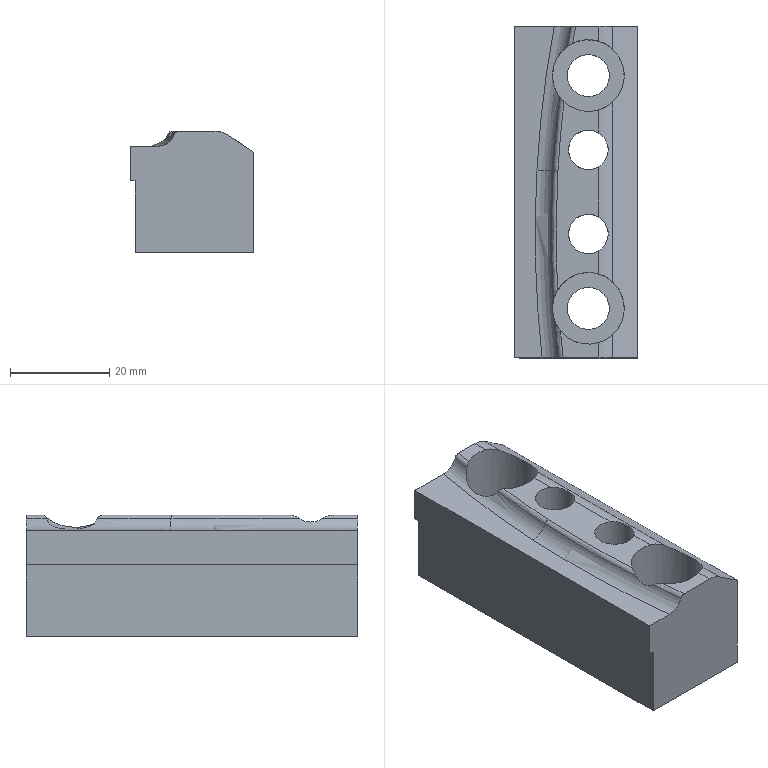Part | NX | features solid 2 | 1 solid | 29 faces | box 25 x 67 x 24.5 mm | volume 29276 mm3 | plane 14 | cylinder 9 | torus 6 | commonest cylinder face diameters 10 x3 8.001 x2 8.5 x2 14.5 x2
STEP:
#1=CARTESIAN_POINT('',(776.878,-36.625,-8.5));
#2=VERTEX_POINT('',#1);
#3=CARTESIAN_POINT('',(776.878,30.375,-8.5));
#4=VERTEX_POINT('',#3);
#5=CARTESIAN_POINT('',(776.878,-3.125,-8.5));
#6=DIRECTION('',(0.,1.,0.));
#7=VECTOR('',#6,1000.);
#8=LINE('',#5,#7);
#9=EDGE_CURVE('',#2,#4,#8,.T.);
#10=ORIENTED_EDGE('',*,*,#9,.F.);
#11=CARTESIAN_POINT('',(775.878,-36.625,-8.5));
#12=VERTEX_POINT('',#11);
#13=CARTESIAN_POINT('',(795.878,-36.625,-8.5));
#14=DIRECTION('',(-1.,0.,0.));
#15=VECTOR('',#14,1000.);
#16=LINE('',#13,#15);
#17=EDGE_CURVE('',#12,#2,#16,.F.);
#18=ORIENTED_EDGE('',*,*,#17,.F.);
#19=CARTESIAN_POINT('',(775.878,30.375,-8.5));
#20=VERTEX_POINT('',#19);
#21=CARTESIAN_POINT('',(775.878,0.7578,-8.5));
#22=DIRECTION('',(0.,-1.,0.));
#23=VECTOR('',#22,1000.);
#24=LINE('',#21,#23);
#25=EDGE_CURVE('',#20,#12,#24,.T.);
#26=ORIENTED_EDGE('',*,*,#25,.F.);
#27=CARTESIAN_POINT('',(795.878,30.375,-8.5));
#28=DIRECTION('',(-1.,0.,0.));
#29=VECTOR('',#28,1000.);
#30=LINE('',#27,#29);
#31=EDGE_CURVE('',#4,#20,#30,.T.);
#32=ORIENTED_EDGE('',*,*,#31,.F.);
#33=EDGE_LOOP('',(#10,#18,#26,#32));
#34=FACE_BOUND('',#33,.T.);
#35=CARTESIAN_POINT('',(779.931,-3.125,-8.5));
#36=DIRECTION('',(0.,0.,1.));
#37=DIRECTION('',(1.,0.,0.));
#38=AXIS2_PLACEMENT_3D('',#35,#36,#37);
#39=PLANE('',#38);
#40=ADVANCED_FACE('',(#34),#39,.F.);
#41=CARTESIAN_POINT('',(785.109,15.984,0.8333));
#42=VERTEX_POINT('',#41);
#43=CARTESIAN_POINT('',(785.947,15.06,1.5));
#44=VERTEX_POINT('',#43);
#45=CARTESIAN_POINT('',(785.109,15.984,0.8333));
#46=CARTESIAN_POINT('',(785.246,15.804,1.28));
#47=CARTESIAN_POINT('',(785.582,15.398,1.5));
#48=CARTESIAN_POINT('',(785.947,15.06,1.5));
#49=B_SPLINE_CURVE_WITH_KNOTS('',3,(#45,#46,#47,#48),.UNSPECIFIED.,.F.,.F.,(4,4),(0.,0.001475),.UNSPECIFIED.);
#50=EDGE_CURVE('',#42,#44,#49,.T.);
#51=ORIENTED_EDGE('',*,*,#50,.F.);
#52=CARTESIAN_POINT('',(783.786,1.121,0.8333));
#53=VERTEX_POINT('',#52);
#54=CARTESIAN_POINT('',(1009.499,-11.474,0.8333));
#55=DIRECTION('',(0.,0.,1.));
#56=DIRECTION('',(1.,0.,0.));
#57=AXIS2_PLACEMENT_3D('',#54,#55,#56);
#58=CIRCLE('',#57,226.064);
#59=EDGE_CURVE('',#53,#42,#58,.F.);
#60=ORIENTED_EDGE('',*,*,#59,.F.);
#61=CARTESIAN_POINT('',(784.727,1.069,1.5));
#62=VERTEX_POINT('',#61);
#63=CARTESIAN_POINT('',(784.727,1.069,0.5));
#64=DIRECTION('',(0.05572,0.9984,0.));
#65=DIRECTION('',(0.9573,-0.05342,0.284));
#66=AXIS2_PLACEMENT_3D('',#63,#64,#65);
#67=CIRCLE('',#66,1.);
#68=EDGE_CURVE('',#62,#53,#67,.F.);
#69=ORIENTED_EDGE('',*,*,#68,.F.);
#70=CARTESIAN_POINT('',(792.133,47.106,1.5));
#71=CARTESIAN_POINT('',(789.702,38.085,1.5));
#72=CARTESIAN_POINT('',(787.739,28.939,1.5));
#73=CARTESIAN_POINT('',(786.252,19.698,1.5));
#74=CARTESIAN_POINT('',(785.248,10.397,1.5));
#75=CARTESIAN_POINT('',(784.727,1.069,1.5));
#76=B_SPLINE_CURVE_WITH_KNOTS('',5,(#70,#71,#72,#73,#74,#75),.UNSPECIFIED.,.F.,.F.,(6,6),(0.,1.),.PIECEWISE_BEZIER_KNOTS.);
#77=EDGE_CURVE('',#62,#44,#76,.F.);
#78=ORIENTED_EDGE('',*,*,#77,.T.);
#79=EDGE_LOOP('',(#51,#60,#69,#78));
#80=FACE_BOUND('',#79,.T.);
#81=CARTESIAN_POINT('',(1009.499,-11.474,0.5));
#82=DIRECTION('',(0.,0.,1.));
#83=DIRECTION('',(-0.9984,0.05572,0.));
#84=AXIS2_PLACEMENT_3D('',#81,#82,#83);
#85=TOROIDAL_SURFACE('',#84,225.121,1.);
#86=ADVANCED_FACE('',(#80),#85,.T.);
#87=ORIENTED_EDGE('',*,*,#59,.T.);
#88=CARTESIAN_POINT('',(786.601,26.23,0.8333));
#89=VERTEX_POINT('',#88);
#90=CARTESIAN_POINT('',(785.109,15.984,0.8333));
#91=CARTESIAN_POINT('',(784.81,16.377,-0.1402));
#92=CARTESIAN_POINT('',(783.709,18.148,-1.214));
#93=CARTESIAN_POINT('',(783.465,21.462,-1.338));
#94=CARTESIAN_POINT('',(784.453,24.019,-1.218));
#95=CARTESIAN_POINT('',(785.782,25.597,-0.448));
#96=CARTESIAN_POINT('',(786.402,26.084,0.3461));
#97=CARTESIAN_POINT('',(786.601,26.23,0.8333));
#98=B_SPLINE_CURVE_WITH_KNOTS('',3,(#90,#91,#92,#93,#94,#95,#96,#97),.UNSPECIFIED.,.F.,.F.,(4,1,1,1,1,4),(0.,0.003217,0.006434,0.009651,0.01126,0.01287),.UNSPECIFIED.);
#99=EDGE_CURVE('',#42,#89,#98,.T.);
#100=ORIENTED_EDGE('',*,*,#99,.T.);
#101=CARTESIAN_POINT('',(787.342,30.375,0.8333));
#102=VERTEX_POINT('',#101);
#103=CARTESIAN_POINT('',(1009.499,-11.474,0.8333));
#104=DIRECTION('',(0.,0.,1.));
#105=DIRECTION('',(1.,0.,0.));
#106=AXIS2_PLACEMENT_3D('',#103,#104,#105);
#107=CIRCLE('',#106,226.064);
#108=EDGE_CURVE('',#89,#102,#107,.F.);
#109=ORIENTED_EDGE('',*,*,#108,.T.);
#110=CARTESIAN_POINT('',(783.985,30.375,-1.5));
#111=VERTEX_POINT('',#110);
#112=CARTESIAN_POINT('',(783.985,30.375,-1.5));
#113=CARTESIAN_POINT('',(785.449,30.375,-1.5));
#114=CARTESIAN_POINT('',(786.846,30.375,-0.5449));
#115=CARTESIAN_POINT('',(787.342,30.375,0.8333));
#116=B_SPLINE_CURVE_WITH_KNOTS('',3,(#112,#113,#114,#115),.UNSPECIFIED.,.F.,.F.,(4,4),(0.,0.00433),.UNSPECIFIED.);
#117=EDGE_CURVE('',#111,#102,#116,.T.);
#118=ORIENTED_EDGE('',*,*,#117,.F.);
#119=CARTESIAN_POINT('',(780.491,1.305,-1.5));
#120=VERTEX_POINT('',#119);
#121=CARTESIAN_POINT('',(788.037,48.21,-1.5));
#122=CARTESIAN_POINT('',(784.94,36.722,-1.5));
#123=CARTESIAN_POINT('',(782.639,25.019,-1.5));
#124=CARTESIAN_POINT('',(781.154,13.185,-1.5));
#125=CARTESIAN_POINT('',(780.491,1.305,-1.5));
#126=B_SPLINE_CURVE_WITH_KNOTS('',4,(#121,#122,#123,#124,#125),.UNSPECIFIED.,.F.,.F.,(5,5),(0.,1.),.PIECEWISE_BEZIER_KNOTS.);
#127=EDGE_CURVE('',#120,#111,#126,.F.);
#128=ORIENTED_EDGE('',*,*,#127,.F.);
#129=CARTESIAN_POINT('',(780.491,1.305,2.));
#130=DIRECTION('',(0.05572,0.9984,0.));
#131=DIRECTION('',(0.9573,-0.05342,0.284));
#132=AXIS2_PLACEMENT_3D('',#129,#130,#131);
#133=CIRCLE('',#132,3.5);
#134=EDGE_CURVE('',#120,#53,#133,.F.);
#135=ORIENTED_EDGE('',*,*,#134,.T.);
#136=EDGE_LOOP('',(#87,#100,#109,#118,#128,#135));
#137=FACE_BOUND('',#136,.T.);
#138=CARTESIAN_POINT('',(1009.499,-11.474,2.));
#139=DIRECTION('',(0.,0.,1.));
#140=DIRECTION('',(-0.9984,0.05572,0.));
#141=AXIS2_PLACEMENT_3D('',#138,#139,#140);
#142=TOROIDAL_SURFACE('',#141,229.364,3.5);
#143=ADVANCED_FACE('',(#137),#142,.F.);
#144=CARTESIAN_POINT('',(787.668,26.876,1.5));
#145=VERTEX_POINT('',#144);
#146=CARTESIAN_POINT('',(787.668,26.876,1.5));
#147=CARTESIAN_POINT('',(787.221,26.655,1.5));
#148=CARTESIAN_POINT('',(786.784,26.363,1.28));
#149=CARTESIAN_POINT('',(786.601,26.23,0.8333));
#150=B_SPLINE_CURVE_WITH_KNOTS('',3,(#146,#147,#148,#149),.UNSPECIFIED.,.F.,.F.,(4,4),(0.,0.001475),.UNSPECIFIED.);
#151=EDGE_CURVE('',#145,#89,#150,.T.);
#152=ORIENTED_EDGE('',*,*,#151,.F.);
#153=CARTESIAN_POINT('',(788.302,30.375,1.5));
#154=VERTEX_POINT('',#153);
#155=CARTESIAN_POINT('',(792.133,47.106,1.5));
#156=CARTESIAN_POINT('',(789.702,38.085,1.5));
#157=CARTESIAN_POINT('',(787.739,28.939,1.5));
#158=CARTESIAN_POINT('',(786.252,19.698,1.5));
#159=CARTESIAN_POINT('',(785.248,10.397,1.5));
#160=CARTESIAN_POINT('',(784.727,1.069,1.5));
#161=B_SPLINE_CURVE_WITH_KNOTS('',5,(#155,#156,#157,#158,#159,#160),.UNSPECIFIED.,.F.,.F.,(6,6),(0.,1.),.PIECEWISE_BEZIER_KNOTS.);
#162=EDGE_CURVE('',#145,#154,#161,.F.);
#163=ORIENTED_EDGE('',*,*,#162,.T.);
#164=CARTESIAN_POINT('',(788.302,30.375,1.5));
#165=CARTESIAN_POINT('',(787.883,30.375,1.5));
#166=CARTESIAN_POINT('',(787.484,30.375,1.227));
#167=CARTESIAN_POINT('',(787.342,30.375,0.8333));
#168=B_SPLINE_CURVE_WITH_KNOTS('',3,(#164,#165,#166,#167),.UNSPECIFIED.,.F.,.F.,(4,4),(0.,0.001238),.UNSPECIFIED.);
#169=EDGE_CURVE('',#154,#102,#168,.T.);
#170=ORIENTED_EDGE('',*,*,#169,.T.);
#171=ORIENTED_EDGE('',*,*,#108,.F.);
#172=EDGE_LOOP('',(#152,#163,#170,#171));
#173=FACE_BOUND('',#172,.T.);
#174=CARTESIAN_POINT('',(1009.499,-11.474,0.5));
#175=DIRECTION('',(0.,0.,1.));
#176=DIRECTION('',(-0.9984,0.05572,0.));
#177=AXIS2_PLACEMENT_3D('',#174,#175,#176);
#178=TOROIDAL_SURFACE('',#177,225.121,1.);
#179=ADVANCED_FACE('',(#173),#178,.T.);
#180=CARTESIAN_POINT('',(793.008,27.305,1.5));
#181=VERTEX_POINT('',#180);
#182=CARTESIAN_POINT('',(793.008,30.375,1.5));
#183=VERTEX_POINT('',#182);
#184=CARTESIAN_POINT('',(793.008,-3.125,1.5));
#185=DIRECTION('',(0.,-1.,0.));
#186=VECTOR('',#185,1000.);
#187=LINE('',#184,#186);
#188=EDGE_CURVE('',#181,#183,#187,.F.);
#189=ORIENTED_EDGE('',*,*,#188,.T.);
#190=CARTESIAN_POINT('',(795.878,30.375,1.5));
#191=DIRECTION('',(-1.,0.,0.));
#192=VECTOR('',#191,1000.);
#193=LINE('',#190,#192);
#194=EDGE_CURVE('',#183,#154,#193,.T.);
#195=ORIENTED_EDGE('',*,*,#194,.T.);
#196=ORIENTED_EDGE('',*,*,#162,.F.);
#197=CARTESIAN_POINT('',(790.878,20.375,1.5));
#198=DIRECTION('',(0.,0.,1.));
#199=DIRECTION('',(1.,0.,0.));
#200=AXIS2_PLACEMENT_3D('',#197,#198,#199);
#201=CIRCLE('',#200,7.25);
#202=EDGE_CURVE('',#181,#145,#201,.T.);
#203=ORIENTED_EDGE('',*,*,#202,.F.);
#204=EDGE_LOOP('',(#189,#195,#196,#203));
#205=FACE_BOUND('',#204,.T.);
#206=CARTESIAN_POINT('',(445.33,343.366,1.5));
#207=DIRECTION('',(0.,0.,1.));
#208=DIRECTION('',(0.,-1.,0.));
#209=AXIS2_PLACEMENT_3D('',#206,#207,#208);
#210=PLANE('',#209);
#211=ADVANCED_FACE('',(#205),#210,.T.);
#212=ORIENTED_EDGE('',*,*,#188,.F.);
#213=CARTESIAN_POINT('',(795.782,25.715,0.6603));
#214=VERTEX_POINT('',#213);
#215=CARTESIAN_POINT('',(793.008,27.305,1.5));
#216=CARTESIAN_POINT('',(794.09,26.972,1.5));
#217=CARTESIAN_POINT('',(795.036,26.399,1.157));
#218=CARTESIAN_POINT('',(795.782,25.715,0.6603));
#219=B_SPLINE_CURVE_WITH_KNOTS('',3,(#215,#216,#217,#218),.UNSPECIFIED.,.F.,.F.,(4,4),(0.,0.003338),.UNSPECIFIED.);
#220=EDGE_CURVE('',#181,#214,#219,.T.);
#221=ORIENTED_EDGE('',*,*,#220,.T.);
#222=CARTESIAN_POINT('',(795.782,30.375,0.6603));
#223=VERTEX_POINT('',#222);
#224=CARTESIAN_POINT('',(795.782,-3.125,0.6603));
#225=DIRECTION('',(0.,-1.,0.));
#226=VECTOR('',#225,1000.);
#227=LINE('',#224,#226);
#228=EDGE_CURVE('',#223,#214,#227,.T.);
#229=ORIENTED_EDGE('',*,*,#228,.F.);
#230=CARTESIAN_POINT('',(793.008,30.375,-3.5));
#231=DIRECTION('',(0.,1.,0.));
#232=DIRECTION('',(0.,0.,1.));
#233=AXIS2_PLACEMENT_3D('',#230,#231,#232);
#234=CIRCLE('',#233,5.);
#235=EDGE_CURVE('',#183,#223,#234,.T.);
#236=ORIENTED_EDGE('',*,*,#235,.F.);
#237=EDGE_LOOP('',(#212,#221,#229,#236));
#238=FACE_BOUND('',#237,.T.);
#239=CARTESIAN_POINT('',(793.008,-3.125,-3.5));
#240=DIRECTION('',(0.,-1.,0.));
#241=DIRECTION('',(0.,0.,-1.));
#242=AXIS2_PLACEMENT_3D('',#239,#240,#241);
#243=CYLINDRICAL_SURFACE('',#242,5.);
#244=ADVANCED_FACE('',(#238),#243,.T.);
#245=CARTESIAN_POINT('',(795.782,-31.965,0.6603));
#246=VERTEX_POINT('',#245);
#247=CARTESIAN_POINT('',(795.782,-36.625,0.6603));
#248=VERTEX_POINT('',#247);
#249=CARTESIAN_POINT('',(795.782,-3.125,0.6603));
#250=DIRECTION('',(0.,-1.,0.));
#251=VECTOR('',#250,1000.);
#252=LINE('',#249,#251);
#253=EDGE_CURVE('',#246,#248,#252,.T.);
#254=ORIENTED_EDGE('',*,*,#253,.F.);
#255=CARTESIAN_POINT('',(793.008,-33.555,1.5));
#256=VERTEX_POINT('',#255);
#257=CARTESIAN_POINT('',(795.782,-31.965,0.6603));
#258=CARTESIAN_POINT('',(795.037,-32.649,1.157));
#259=CARTESIAN_POINT('',(794.09,-33.222,1.5));
#260=CARTESIAN_POINT('',(793.008,-33.555,1.5));
#261=B_SPLINE_CURVE_WITH_KNOTS('',3,(#257,#258,#259,#260),.UNSPECIFIED.,.F.,.F.,(4,4),(0.,0.003342),.UNSPECIFIED.);
#262=EDGE_CURVE('',#246,#256,#261,.T.);
#263=ORIENTED_EDGE('',*,*,#262,.T.);
#264=CARTESIAN_POINT('',(793.008,-36.625,1.5));
#265=VERTEX_POINT('',#264);
#266=CARTESIAN_POINT('',(793.008,-3.125,1.5));
#267=DIRECTION('',(0.,-1.,0.));
#268=VECTOR('',#267,1000.);
#269=LINE('',#266,#268);
#270=EDGE_CURVE('',#265,#256,#269,.F.);
#271=ORIENTED_EDGE('',*,*,#270,.F.);
#272=CARTESIAN_POINT('',(793.008,-36.625,-3.5));
#273=DIRECTION('',(0.,-1.,0.));
#274=DIRECTION('',(0.,0.,-1.));
#275=AXIS2_PLACEMENT_3D('',#272,#273,#274);
#276=CIRCLE('',#275,5.);
#277=EDGE_CURVE('',#248,#265,#276,.T.);
#278=ORIENTED_EDGE('',*,*,#277,.F.);
#279=EDGE_LOOP('',(#254,#263,#271,#278));
#280=FACE_BOUND('',#279,.T.);
#281=CARTESIAN_POINT('',(793.008,-3.125,-3.5));
#282=DIRECTION('',(0.,-1.,0.));
#283=DIRECTION('',(0.,0.,-1.));
#284=AXIS2_PLACEMENT_3D('',#281,#282,#283);
#285=CYLINDRICAL_SURFACE('',#284,5.);
#286=ADVANCED_FACE('',(#280),#285,.T.);
#287=ORIENTED_EDGE('',*,*,#270,.T.);
#288=CARTESIAN_POINT('',(785.242,-31.186,1.5));
#289=VERTEX_POINT('',#288);
#290=CARTESIAN_POINT('',(790.878,-26.625,1.5));
#291=DIRECTION('',(0.,0.,1.));
#292=DIRECTION('',(1.,0.,0.));
#293=AXIS2_PLACEMENT_3D('',#290,#291,#292);
#294=CIRCLE('',#293,7.25);
#295=EDGE_CURVE('',#289,#256,#294,.T.);
#296=ORIENTED_EDGE('',*,*,#295,.F.);
#297=CARTESIAN_POINT('',(785.787,-36.625,1.5));
#298=VERTEX_POINT('',#297);
#299=CARTESIAN_POINT('',(784.727,1.069,1.5));
#300=CARTESIAN_POINT('',(784.207,-8.259,1.5));
#301=CARTESIAN_POINT('',(784.17,-17.615,1.5));
#302=CARTESIAN_POINT('',(784.619,-26.963,1.5));
#303=CARTESIAN_POINT('',(785.553,-36.272,1.5));
#304=CARTESIAN_POINT('',(786.965,-45.507,1.5));
#305=B_SPLINE_CURVE_WITH_KNOTS('',5,(#299,#300,#301,#302,#303,#304),.UNSPECIFIED.,.F.,.F.,(6,6),(0.,1.),.PIECEWISE_BEZIER_KNOTS.);
#306=EDGE_CURVE('',#298,#289,#305,.F.);
#307=ORIENTED_EDGE('',*,*,#306,.F.);
#308=CARTESIAN_POINT('',(795.878,-36.625,1.5));
#309=DIRECTION('',(-1.,0.,0.));
#310=VECTOR('',#309,1000.);
#311=LINE('',#308,#310);
#312=EDGE_CURVE('',#265,#298,#311,.T.);
#313=ORIENTED_EDGE('',*,*,#312,.F.);
#314=EDGE_LOOP('',(#287,#296,#307,#313));
#315=FACE_BOUND('',#314,.T.);
#316=CARTESIAN_POINT('',(445.33,343.366,1.5));
#317=DIRECTION('',(0.,0.,1.));
#318=DIRECTION('',(0.,-1.,0.));
#319=AXIS2_PLACEMENT_3D('',#316,#317,#318);
#320=PLANE('',#319);
#321=ADVANCED_FACE('',(#315),#320,.T.);
#322=CARTESIAN_POINT('',(784.139,-29.298,0.8333));
#323=VERTEX_POINT('',#322);
#324=CARTESIAN_POINT('',(784.139,-29.298,0.8333));
#325=CARTESIAN_POINT('',(784.25,-29.58,1.086));
#326=CARTESIAN_POINT('',(784.565,-30.253,1.358));
#327=CARTESIAN_POINT('',(784.998,-30.885,1.5));
#328=CARTESIAN_POINT('',(785.242,-31.186,1.5));
#329=B_SPLINE_CURVE_WITH_KNOTS('',3,(#324,#325,#326,#327,#328),.UNSPECIFIED.,.F.,.F.,(4,1,4),(0.000000307,0.001165,0.002329),.UNSPECIFIED.);
#330=EDGE_CURVE('',#323,#289,#329,.T.);
#331=ORIENTED_EDGE('',*,*,#330,.F.);
#332=CARTESIAN_POINT('',(784.838,-36.625,0.8333));
#333=VERTEX_POINT('',#332);
#334=CARTESIAN_POINT('',(1009.499,-11.474,0.8333));
#335=DIRECTION('',(0.,0.,1.));
#336=DIRECTION('',(1.,0.,0.));
#337=AXIS2_PLACEMENT_3D('',#334,#335,#336);
#338=CIRCLE('',#337,226.064);
#339=EDGE_CURVE('',#333,#323,#338,.F.);
#340=ORIENTED_EDGE('',*,*,#339,.F.);
#341=CARTESIAN_POINT('',(785.787,-36.625,1.5));
#342=CARTESIAN_POINT('',(785.376,-36.625,1.5));
#343=CARTESIAN_POINT('',(784.976,-36.625,1.22));
#344=CARTESIAN_POINT('',(784.838,-36.625,0.8333));
#345=B_SPLINE_CURVE_WITH_KNOTS('',3,(#341,#342,#343,#344),.UNSPECIFIED.,.F.,.F.,(4,4),(0.00528,0.006509),.UNSPECIFIED.);
#346=EDGE_CURVE('',#298,#333,#345,.T.);
#347=ORIENTED_EDGE('',*,*,#346,.F.);
#348=ORIENTED_EDGE('',*,*,#306,.T.);
#349=EDGE_LOOP('',(#331,#340,#347,#348));
#350=FACE_BOUND('',#349,.T.);
#351=CARTESIAN_POINT('',(1009.499,-11.474,0.5));
#352=DIRECTION('',(0.,0.,1.));
#353=DIRECTION('',(0.9984,-0.05572,0.));
#354=AXIS2_PLACEMENT_3D('',#351,#352,#353);
#355=TOROIDAL_SURFACE('',#354,225.121,1.);
#356=ADVANCED_FACE('',(#350),#355,.T.);
#357=ORIENTED_EDGE('',*,*,#339,.T.);
#358=CARTESIAN_POINT('',(783.834,-24.906,0.8333));
#359=VERTEX_POINT('',#358);
#360=CARTESIAN_POINT('',(784.139,-29.298,0.8333));
#361=CARTESIAN_POINT('',(783.91,-28.723,0.318));
#362=CARTESIAN_POINT('',(783.491,-27.14,-0.02762));
#363=CARTESIAN_POINT('',(783.688,-25.506,0.3192));
#364=CARTESIAN_POINT('',(783.834,-24.906,0.8333));
#365=B_SPLINE_CURVE_WITH_KNOTS('',3,(#360,#361,#362,#363,#364),.UNSPECIFIED.,.F.,.F.,(4,1,4),(0.000000306,0.002366,0.004731),.UNSPECIFIED.);
#366=EDGE_CURVE('',#323,#359,#365,.T.);
#367=ORIENTED_EDGE('',*,*,#366,.T.);
#368=CARTESIAN_POINT('',(1009.499,-11.474,0.8333));
#369=DIRECTION('',(0.,0.,1.));
#370=DIRECTION('',(1.,0.,0.));
#371=AXIS2_PLACEMENT_3D('',#368,#369,#370);
#372=CIRCLE('',#371,226.064);
#373=EDGE_CURVE('',#359,#53,#372,.F.);
#374=ORIENTED_EDGE('',*,*,#373,.T.);
#375=ORIENTED_EDGE('',*,*,#134,.F.);
#376=CARTESIAN_POINT('',(781.518,-36.625,-1.5));
#377=VERTEX_POINT('',#376);
#378=CARTESIAN_POINT('',(1009.499,-11.474,-1.5));
#379=DIRECTION('',(0.,0.,1.));
#380=DIRECTION('',(1.,0.,0.));
#381=AXIS2_PLACEMENT_3D('',#378,#379,#380);
#382=CIRCLE('',#381,229.364);
#383=EDGE_CURVE('',#377,#120,#382,.F.);
#384=ORIENTED_EDGE('',*,*,#383,.F.);
#385=CARTESIAN_POINT('',(781.518,-36.625,-1.5));
#386=CARTESIAN_POINT('',(782.959,-36.625,-1.5));
#387=CARTESIAN_POINT('',(784.357,-36.625,-0.5186));
#388=CARTESIAN_POINT('',(784.838,-36.625,0.8333));
#389=B_SPLINE_CURVE_WITH_KNOTS('',3,(#385,#386,#387,#388),.UNSPECIFIED.,.F.,.F.,(4,4),(0.0009387,0.005242),.UNSPECIFIED.);
#390=EDGE_CURVE('',#377,#333,#389,.T.);
#391=ORIENTED_EDGE('',*,*,#390,.T.);
#392=EDGE_LOOP('',(#357,#367,#374,#375,#384,#391));
#393=FACE_BOUND('',#392,.T.);
#394=CARTESIAN_POINT('',(1009.499,-11.474,2.));
#395=DIRECTION('',(0.,0.,1.));
#396=DIRECTION('',(0.9984,-0.05572,0.));
#397=AXIS2_PLACEMENT_3D('',#394,#395,#396);
#398=TOROIDAL_SURFACE('',#397,229.364,3.5);
#399=ADVANCED_FACE('',(#393),#398,.F.);
#400=CARTESIAN_POINT('',(784.667,-22.884,1.5));
#401=VERTEX_POINT('',#400);
#402=CARTESIAN_POINT('',(784.667,-22.884,1.5));
#403=CARTESIAN_POINT('',(784.467,-23.216,1.5));
#404=CARTESIAN_POINT('',(784.124,-23.904,1.358));
#405=CARTESIAN_POINT('',(783.906,-24.613,1.085));
#406=CARTESIAN_POINT('',(783.834,-24.906,0.8333));
#407=B_SPLINE_CURVE_WITH_KNOTS('',3,(#402,#403,#404,#405,#406),.UNSPECIFIED.,.F.,.F.,(4,1,4),(0.0017,0.002868,0.004036),.UNSPECIFIED.);
#408=EDGE_CURVE('',#401,#359,#407,.T.);
#409=ORIENTED_EDGE('',*,*,#408,.F.);
#410=CARTESIAN_POINT('',(784.727,1.069,1.5));
#411=CARTESIAN_POINT('',(784.207,-8.259,1.5));
#412=CARTESIAN_POINT('',(784.17,-17.615,1.5));
#413=CARTESIAN_POINT('',(784.619,-26.963,1.5));
#414=CARTESIAN_POINT('',(785.553,-36.272,1.5));
#415=CARTESIAN_POINT('',(786.965,-45.507,1.5));
#416=B_SPLINE_CURVE_WITH_KNOTS('',5,(#410,#411,#412,#413,#414,#415),.UNSPECIFIED.,.F.,.F.,(6,6),(0.,1.),.PIECEWISE_BEZIER_KNOTS.);
#417=EDGE_CURVE('',#401,#62,#416,.F.);
#418=ORIENTED_EDGE('',*,*,#417,.T.);
#419=ORIENTED_EDGE('',*,*,#68,.T.);
#420=ORIENTED_EDGE('',*,*,#373,.F.);
#421=EDGE_LOOP('',(#409,#418,#419,#420));
#422=FACE_BOUND('',#421,.T.);
#423=CARTESIAN_POINT('',(1009.499,-11.474,0.5));
#424=DIRECTION('',(0.,0.,1.));
#425=DIRECTION('',(0.9984,-0.05572,0.));
#426=AXIS2_PLACEMENT_3D('',#423,#424,#425);
#427=TOROIDAL_SURFACE('',#426,225.121,1.);
#428=ADVANCED_FACE('',(#422),#427,.T.);
#429=CARTESIAN_POINT('',(793.008,8.761,1.5));
#430=VERTEX_POINT('',#429);
#431=CARTESIAN_POINT('',(793.008,13.445,1.5));
#432=VERTEX_POINT('',#431);
#433=CARTESIAN_POINT('',(793.008,-3.125,1.5));
#434=DIRECTION('',(0.,-1.,0.));
#435=VECTOR('',#434,1000.);
#436=LINE('',#433,#435);
#437=EDGE_CURVE('',#430,#432,#436,.F.);
#438=ORIENTED_EDGE('',*,*,#437,.T.);
#439=CARTESIAN_POINT('',(790.878,20.375,1.5));
#440=DIRECTION('',(0.,0.,1.));
#441=DIRECTION('',(1.,0.,0.));
#442=AXIS2_PLACEMENT_3D('',#439,#440,#441);
#443=CIRCLE('',#442,7.25);
#444=EDGE_CURVE('',#44,#432,#443,.T.);
#445=ORIENTED_EDGE('',*,*,#444,.F.);
#446=ORIENTED_EDGE('',*,*,#77,.F.);
#447=ORIENTED_EDGE('',*,*,#417,.F.);
#448=CARTESIAN_POINT('',(793.008,-19.695,1.5));
#449=VERTEX_POINT('',#448);
#450=CARTESIAN_POINT('',(790.878,-26.625,1.5));
#451=DIRECTION('',(0.,0.,1.));
#452=DIRECTION('',(1.,0.,0.));
#453=AXIS2_PLACEMENT_3D('',#450,#451,#452);
#454=CIRCLE('',#453,7.25);
#455=EDGE_CURVE('',#449,#401,#454,.T.);
#456=ORIENTED_EDGE('',*,*,#455,.F.);
#457=CARTESIAN_POINT('',(793.008,-15.011,1.5));
#458=VERTEX_POINT('',#457);
#459=CARTESIAN_POINT('',(793.008,-3.125,1.5));
#460=DIRECTION('',(0.,-1.,0.));
#461=VECTOR('',#460,1000.);
#462=LINE('',#459,#461);
#463=EDGE_CURVE('',#449,#458,#462,.F.);
#464=ORIENTED_EDGE('',*,*,#463,.T.);
#465=CARTESIAN_POINT('',(793.008,-8.239,1.5));
#466=VERTEX_POINT('',#465);
#467=CARTESIAN_POINT('',(790.878,-11.625,1.5));
#468=DIRECTION('',(0.,0.,1.));
#469=DIRECTION('',(1.,0.,0.));
#470=AXIS2_PLACEMENT_3D('',#467,#468,#469);
#471=CIRCLE('',#470,4.);
#472=EDGE_CURVE('',#466,#458,#471,.T.);
#473=ORIENTED_EDGE('',*,*,#472,.F.);
#474=CARTESIAN_POINT('',(793.008,1.989,1.5));
#475=VERTEX_POINT('',#474);
#476=CARTESIAN_POINT('',(793.008,-3.125,1.5));
#477=DIRECTION('',(0.,-1.,0.));
#478=VECTOR('',#477,1000.);
#479=LINE('',#476,#478);
#480=EDGE_CURVE('',#466,#475,#479,.F.);
#481=ORIENTED_EDGE('',*,*,#480,.T.);
#482=CARTESIAN_POINT('',(790.878,5.375,1.5));
#483=DIRECTION('',(0.,0.,1.));
#484=DIRECTION('',(1.,0.,0.));
#485=AXIS2_PLACEMENT_3D('',#482,#483,#484);
#486=CIRCLE('',#485,4.);
#487=EDGE_CURVE('',#430,#475,#486,.T.);
#488=ORIENTED_EDGE('',*,*,#487,.F.);
#489=EDGE_LOOP('',(#438,#445,#446,#447,#456,#464,#473,#481,#488));
#490=FACE_BOUND('',#489,.T.);
#491=CARTESIAN_POINT('',(445.33,343.366,1.5));
#492=DIRECTION('',(0.,0.,1.));
#493=DIRECTION('',(0.,-1.,0.));
#494=AXIS2_PLACEMENT_3D('',#491,#492,#493);
#495=PLANE('',#494);
#496=ADVANCED_FACE('',(#490),#495,.T.);
#497=CARTESIAN_POINT('',(793.008,-8.239,1.5));
#498=CARTESIAN_POINT('',(794.165,-8.967,1.5));
#499=CARTESIAN_POINT('',(795.591,-11.622,0.7743));
#500=CARTESIAN_POINT('',(794.165,-14.283,1.5));
#501=CARTESIAN_POINT('',(793.008,-15.011,1.5));
#502=B_SPLINE_CURVE_WITH_KNOTS('',3,(#497,#498,#499,#500,#501),.UNSPECIFIED.,.F.,.F.,(4,1,4),(0.,0.004035,0.008069),.UNSPECIFIED.);
#503=EDGE_CURVE('',#466,#458,#502,.T.);
#504=ORIENTED_EDGE('',*,*,#503,.F.);
#505=ORIENTED_EDGE('',*,*,#472,.T.);
#506=EDGE_LOOP('',(#504,#505));
#507=FACE_BOUND('',#506,.T.);
#508=CARTESIAN_POINT('',(786.877,-11.625,-23.));
#509=VERTEX_POINT('',#508);
#510=CARTESIAN_POINT('',(790.878,-11.625,-23.));
#511=DIRECTION('',(0.,0.,-1.));
#512=DIRECTION('',(-1.,0.,0.));
#513=AXIS2_PLACEMENT_3D('',#510,#511,#512);
#514=CIRCLE('',#513,4.);
#515=EDGE_CURVE('',#509,#509,#514,.T.);
#516=ORIENTED_EDGE('',*,*,#515,.T.);
#517=EDGE_LOOP('',(#516));
#518=FACE_BOUND('',#517,.T.);
#519=CARTESIAN_POINT('',(790.878,-11.625,37.));
#520=DIRECTION('',(0.,0.,-1.));
#521=DIRECTION('',(-1.,0.,0.));
#522=AXIS2_PLACEMENT_3D('',#519,#520,#521);
#523=CYLINDRICAL_SURFACE('',#522,4.);
#524=ADVANCED_FACE('',(#507,#518),#523,.F.);
#525=CARTESIAN_POINT('',(793.008,8.761,1.5));
#526=CARTESIAN_POINT('',(794.165,8.033,1.5));
#527=CARTESIAN_POINT('',(795.591,5.378,0.7743));
#528=CARTESIAN_POINT('',(794.165,2.717,1.5));
#529=CARTESIAN_POINT('',(793.008,1.989,1.5));
#530=B_SPLINE_CURVE_WITH_KNOTS('',3,(#525,#526,#527,#528,#529),.UNSPECIFIED.,.F.,.F.,(4,1,4),(0.,0.004035,0.008069),.UNSPECIFIED.);
#531=EDGE_CURVE('',#430,#475,#530,.T.);
#532=ORIENTED_EDGE('',*,*,#531,.F.);
#533=ORIENTED_EDGE('',*,*,#487,.T.);
#534=EDGE_LOOP('',(#532,#533));
#535=FACE_BOUND('',#534,.T.);
#536=CARTESIAN_POINT('',(786.877,5.375,-23.));
#537=VERTEX_POINT('',#536);
#538=CARTESIAN_POINT('',(790.878,5.375,-23.));
#539=DIRECTION('',(0.,0.,-1.));
#540=DIRECTION('',(-1.,0.,0.));
#541=AXIS2_PLACEMENT_3D('',#538,#539,#540);
#542=CIRCLE('',#541,4.);
#543=EDGE_CURVE('',#537,#537,#542,.T.);
#544=ORIENTED_EDGE('',*,*,#543,.T.);
#545=EDGE_LOOP('',(#544));
#546=FACE_BOUND('',#545,.T.);
#547=CARTESIAN_POINT('',(790.878,5.375,37.));
#548=DIRECTION('',(0.,0.,-1.));
#549=DIRECTION('',(-1.,0.,0.));
#550=AXIS2_PLACEMENT_3D('',#547,#548,#549);
#551=CYLINDRICAL_SURFACE('',#550,4.);
#552=ADVANCED_FACE('',(#535,#546),#551,.F.);
#553=CARTESIAN_POINT('',(795.782,15.035,0.6603));
#554=VERTEX_POINT('',#553);
#555=CARTESIAN_POINT('',(795.782,-21.285,0.6603));
#556=VERTEX_POINT('',#555);
#557=CARTESIAN_POINT('',(795.782,-3.125,0.6603));
#558=DIRECTION('',(0.,-1.,0.));
#559=VECTOR('',#558,1000.);
#560=LINE('',#557,#559);
#561=EDGE_CURVE('',#554,#556,#560,.T.);
#562=ORIENTED_EDGE('',*,*,#561,.F.);
#563=CARTESIAN_POINT('',(795.782,15.035,0.6603));
#564=CARTESIAN_POINT('',(795.037,14.351,1.157));
#565=CARTESIAN_POINT('',(794.09,13.778,1.5));
#566=CARTESIAN_POINT('',(793.008,13.445,1.5));
#567=B_SPLINE_CURVE_WITH_KNOTS('',3,(#563,#564,#565,#566),.UNSPECIFIED.,.F.,.F.,(4,4),(0.,0.003342),.UNSPECIFIED.);
#568=EDGE_CURVE('',#554,#432,#567,.T.);
#569=ORIENTED_EDGE('',*,*,#568,.T.);
#570=ORIENTED_EDGE('',*,*,#437,.F.);
#571=ORIENTED_EDGE('',*,*,#531,.T.);
#572=ORIENTED_EDGE('',*,*,#480,.F.);
#573=ORIENTED_EDGE('',*,*,#503,.T.);
#574=ORIENTED_EDGE('',*,*,#463,.F.);
#575=CARTESIAN_POINT('',(793.008,-19.695,1.5));
#576=CARTESIAN_POINT('',(794.09,-20.028,1.5));
#577=CARTESIAN_POINT('',(795.036,-20.601,1.157));
#578=CARTESIAN_POINT('',(795.782,-21.285,0.6603));
#579=B_SPLINE_CURVE_WITH_KNOTS('',3,(#575,#576,#577,#578),.UNSPECIFIED.,.F.,.F.,(4,4),(0.,0.003338),.UNSPECIFIED.);
#580=EDGE_CURVE('',#449,#556,#579,.T.);
#581=ORIENTED_EDGE('',*,*,#580,.T.);
#582=EDGE_LOOP('',(#562,#569,#570,#571,#572,#573,#574,#581));
#583=FACE_BOUND('',#582,.T.);
#584=CARTESIAN_POINT('',(793.008,-3.125,-3.5));
#585=DIRECTION('',(0.,-1.,0.));
#586=DIRECTION('',(0.,0.,-1.));
#587=AXIS2_PLACEMENT_3D('',#584,#585,#586);
#588=CYLINDRICAL_SURFACE('',#587,5.);
#589=ADVANCED_FACE('',(#583),#588,.T.);
#590=ORIENTED_EDGE('',*,*,#580,.F.);
#591=ORIENTED_EDGE('',*,*,#455,.T.);
#592=ORIENTED_EDGE('',*,*,#408,.T.);
#593=ORIENTED_EDGE('',*,*,#366,.F.);
#594=ORIENTED_EDGE('',*,*,#330,.T.);
#595=ORIENTED_EDGE('',*,*,#295,.T.);
#596=ORIENTED_EDGE('',*,*,#262,.F.);
#597=CARTESIAN_POINT('',(790.878,-26.625,3.93));
#598=DIRECTION('',(0.5547,0.,0.8321));
#599=DIRECTION('',(0.8321,0.,-0.5547));
#600=AXIS2_PLACEMENT_3D('',#597,#598,#599);
#601=ELLIPSE('',#600,8.713,7.25);
#602=EDGE_CURVE('',#556,#246,#601,.F.);
#603=ORIENTED_EDGE('',*,*,#602,.F.);
#604=EDGE_LOOP('',(#590,#591,#592,#593,#594,#595,#596,#603));
#605=FACE_BOUND('',#604,.T.);
#606=CARTESIAN_POINT('',(783.628,-26.625,-13.));
#607=VERTEX_POINT('',#606);
#608=CARTESIAN_POINT('',(790.878,-26.625,-13.));
#609=DIRECTION('',(0.,0.,-1.));
#610=DIRECTION('',(-1.,0.,0.));
#611=AXIS2_PLACEMENT_3D('',#608,#609,#610);
#612=CIRCLE('',#611,7.25);
#613=EDGE_CURVE('',#607,#607,#612,.F.);
#614=ORIENTED_EDGE('',*,*,#613,.F.);
#615=EDGE_LOOP('',(#614));
#616=FACE_BOUND('',#615,.T.);
#617=CARTESIAN_POINT('',(790.878,-26.625,-1.));
#618=DIRECTION('',(0.,0.,-1.));
#619=DIRECTION('',(1.,0.,0.));
#620=AXIS2_PLACEMENT_3D('',#617,#618,#619);
#621=CYLINDRICAL_SURFACE('',#620,7.25);
#622=ADVANCED_FACE('',(#605,#616),#621,.F.);
#623=ORIENTED_EDGE('',*,*,#220,.F.);
#624=ORIENTED_EDGE('',*,*,#202,.T.);
#625=ORIENTED_EDGE('',*,*,#151,.T.);
#626=ORIENTED_EDGE('',*,*,#99,.F.);
#627=ORIENTED_EDGE('',*,*,#50,.T.);
#628=ORIENTED_EDGE('',*,*,#444,.T.);
#629=ORIENTED_EDGE('',*,*,#568,.F.);
#630=CARTESIAN_POINT('',(790.878,20.375,3.93));
#631=DIRECTION('',(0.5547,0.,0.8321));
#632=DIRECTION('',(0.8321,0.,-0.5547));
#633=AXIS2_PLACEMENT_3D('',#630,#631,#632);
#634=ELLIPSE('',#633,8.713,7.25);
#635=EDGE_CURVE('',#554,#214,#634,.T.);
#636=ORIENTED_EDGE('',*,*,#635,.T.);
#637=EDGE_LOOP('',(#623,#624,#625,#626,#627,#628,#629,#636));
#638=FACE_BOUND('',#637,.T.);
#639=CARTESIAN_POINT('',(783.628,20.375,-13.));
#640=VERTEX_POINT('',#639);
#641=CARTESIAN_POINT('',(790.878,20.375,-13.));
#642=DIRECTION('',(0.,0.,-1.));
#643=DIRECTION('',(-1.,0.,0.));
#644=AXIS2_PLACEMENT_3D('',#641,#642,#643);
#645=CIRCLE('',#644,7.25);
#646=EDGE_CURVE('',#640,#640,#645,.T.);
#647=ORIENTED_EDGE('',*,*,#646,.T.);
#648=EDGE_LOOP('',(#647));
#649=FACE_BOUND('',#648,.T.);
#650=CARTESIAN_POINT('',(790.878,20.375,-1.));
#651=DIRECTION('',(0.,0.,-1.));
#652=DIRECTION('',(1.,0.,0.));
#653=AXIS2_PLACEMENT_3D('',#650,#651,#652);
#654=CYLINDRICAL_SURFACE('',#653,7.25);
#655=ADVANCED_FACE('',(#638,#649),#654,.F.);
#656=CARTESIAN_POINT('',(800.878,30.375,-2.737));
#657=VERTEX_POINT('',#656);
#658=CARTESIAN_POINT('',(796.153,30.375,0.4128));
#659=DIRECTION('',(-0.8321,0.,0.5547));
#660=VECTOR('',#659,1000.);
#661=LINE('',#658,#660);
#662=EDGE_CURVE('',#657,#223,#661,.T.);
#663=ORIENTED_EDGE('',*,*,#662,.T.);
#664=ORIENTED_EDGE('',*,*,#228,.T.);
#665=ORIENTED_EDGE('',*,*,#635,.F.);
#666=ORIENTED_EDGE('',*,*,#561,.T.);
#667=ORIENTED_EDGE('',*,*,#602,.T.);
#668=ORIENTED_EDGE('',*,*,#253,.T.);
#669=CARTESIAN_POINT('',(800.878,-36.625,-2.737));
#670=VERTEX_POINT('',#669);
#671=CARTESIAN_POINT('',(786.922,-36.625,6.567));
#672=DIRECTION('',(-0.8321,0.,0.5547));
#673=VECTOR('',#672,1000.);
#674=LINE('',#671,#673);
#675=EDGE_CURVE('',#670,#248,#674,.T.);
#676=ORIENTED_EDGE('',*,*,#675,.F.);
#677=CARTESIAN_POINT('',(800.878,0.7578,-2.737));
#678=DIRECTION('',(0.,-1.,0.));
#679=VECTOR('',#678,1000.);
#680=LINE('',#677,#679);
#681=EDGE_CURVE('',#657,#670,#680,.T.);
#682=ORIENTED_EDGE('',*,*,#681,.F.);
#683=EDGE_LOOP('',(#663,#664,#665,#666,#667,#668,#676,#682));
#684=FACE_BOUND('',#683,.T.);
#685=CARTESIAN_POINT('',(814.268,-3.125,-11.664));
#686=DIRECTION('',(0.5547,0.,0.8321));
#687=DIRECTION('',(0.8321,0.,-0.5547));
#688=AXIS2_PLACEMENT_3D('',#685,#686,#687);
#689=PLANE('',#688);
#690=ADVANCED_FACE('',(#684),#689,.T.);
#691=CARTESIAN_POINT('',(775.878,30.375,-1.5));
#692=VERTEX_POINT('',#691);
#693=CARTESIAN_POINT('',(795.878,30.375,-1.5));
#694=DIRECTION('',(-1.,0.,0.));
#695=VECTOR('',#694,1000.);
#696=LINE('',#693,#695);
#697=EDGE_CURVE('',#111,#692,#696,.T.);
#698=ORIENTED_EDGE('',*,*,#697,.T.);
#699=CARTESIAN_POINT('',(775.878,-36.625,-1.5));
#700=VERTEX_POINT('',#699);
#701=CARTESIAN_POINT('',(775.878,14.172,-1.5));
#702=DIRECTION('',(0.,-1.,0.));
#703=VECTOR('',#702,1000.);
#704=LINE('',#701,#703);
#705=EDGE_CURVE('',#692,#700,#704,.T.);
#706=ORIENTED_EDGE('',*,*,#705,.T.);
#707=CARTESIAN_POINT('',(795.878,-36.625,-1.5));
#708=DIRECTION('',(-1.,0.,0.));
#709=VECTOR('',#708,1000.);
#710=LINE('',#707,#709);
#711=EDGE_CURVE('',#377,#700,#710,.T.);
#712=ORIENTED_EDGE('',*,*,#711,.F.);
#713=ORIENTED_EDGE('',*,*,#383,.T.);
#714=ORIENTED_EDGE('',*,*,#127,.T.);
#715=EDGE_LOOP('',(#698,#706,#712,#713,#714));
#716=FACE_BOUND('',#715,.T.);
#717=CARTESIAN_POINT('',(445.33,343.366,-1.5));
#718=DIRECTION('',(0.,0.,1.));
#719=DIRECTION('',(0.,-1.,0.));
#720=AXIS2_PLACEMENT_3D('',#717,#718,#719);
#721=PLANE('',#720);
#722=ADVANCED_FACE('',(#716),#721,.T.);
#723=CARTESIAN_POINT('',(775.878,30.375,0.));
#724=DIRECTION('',(0.,0.,1.));
#725=VECTOR('',#724,1000.);
#726=LINE('',#723,#725);
#727=EDGE_CURVE('',#20,#692,#726,.T.);
#728=ORIENTED_EDGE('',*,*,#727,.F.);
#729=ORIENTED_EDGE('',*,*,#25,.T.);
#730=CARTESIAN_POINT('',(775.878,-36.625,20.));
#731=DIRECTION('',(0.,0.,1.));
#732=VECTOR('',#731,1000.);
#733=LINE('',#730,#732);
#734=EDGE_CURVE('',#12,#700,#733,.T.);
#735=ORIENTED_EDGE('',*,*,#734,.T.);
#736=ORIENTED_EDGE('',*,*,#705,.F.);
#737=EDGE_LOOP('',(#728,#729,#735,#736));
#738=FACE_BOUND('',#737,.T.);
#739=CARTESIAN_POINT('',(775.878,0.7578,0.));
#740=DIRECTION('',(1.,0.,0.));
#741=DIRECTION('',(0.,0.,-1.));
#742=AXIS2_PLACEMENT_3D('',#739,#740,#741);
#743=PLANE('',#742);
#744=ADVANCED_FACE('',(#738),#743,.F.);
#745=CARTESIAN_POINT('',(800.878,-36.625,-23.));
#746=VERTEX_POINT('',#745);
#747=CARTESIAN_POINT('',(800.878,-36.625,20.));
#748=DIRECTION('',(0.,0.,1.));
#749=VECTOR('',#748,1000.);
#750=LINE('',#747,#749);
#751=EDGE_CURVE('',#746,#670,#750,.T.);
#752=ORIENTED_EDGE('',*,*,#751,.F.);
#753=CARTESIAN_POINT('',(800.878,30.375,-23.));
#754=VERTEX_POINT('',#753);
#755=CARTESIAN_POINT('',(800.878,0.,-23.));
#756=DIRECTION('',(0.,-1.,0.));
#757=VECTOR('',#756,1000.);
#758=LINE('',#755,#757);
#759=EDGE_CURVE('',#754,#746,#758,.T.);
#760=ORIENTED_EDGE('',*,*,#759,.F.);
#761=CARTESIAN_POINT('',(800.878,30.375,0.));
#762=DIRECTION('',(0.,0.,1.));
#763=VECTOR('',#762,1000.);
#764=LINE('',#761,#763);
#765=EDGE_CURVE('',#754,#657,#764,.T.);
#766=ORIENTED_EDGE('',*,*,#765,.T.);
#767=ORIENTED_EDGE('',*,*,#681,.T.);
#768=EDGE_LOOP('',(#752,#760,#766,#767));
#769=FACE_BOUND('',#768,.T.);
#770=CARTESIAN_POINT('',(800.878,0.7578,0.));
#771=DIRECTION('',(1.,0.,0.));
#772=DIRECTION('',(0.,0.,-1.));
#773=AXIS2_PLACEMENT_3D('',#770,#771,#772);
#774=PLANE('',#773);
#775=ADVANCED_FACE('',(#769),#774,.T.);
#776=ORIENTED_EDGE('',*,*,#765,.F.);
#777=CARTESIAN_POINT('',(776.878,30.375,-23.));
#778=VERTEX_POINT('',#777);
#779=CARTESIAN_POINT('',(699.237,30.375,-23.));
#780=DIRECTION('',(-1.,0.,0.));
#781=VECTOR('',#780,1000.);
#782=LINE('',#779,#781);
#783=EDGE_CURVE('',#754,#778,#782,.T.);
#784=ORIENTED_EDGE('',*,*,#783,.T.);
#785=CARTESIAN_POINT('',(776.878,30.375,0.));
#786=DIRECTION('',(0.,0.,1.));
#787=VECTOR('',#786,1000.);
#788=LINE('',#785,#787);
#789=EDGE_CURVE('',#778,#4,#788,.T.);
#790=ORIENTED_EDGE('',*,*,#789,.T.);
#791=ORIENTED_EDGE('',*,*,#31,.T.);
#792=ORIENTED_EDGE('',*,*,#727,.T.);
#793=ORIENTED_EDGE('',*,*,#697,.F.);
#794=ORIENTED_EDGE('',*,*,#117,.T.);
#795=ORIENTED_EDGE('',*,*,#169,.F.);
#796=ORIENTED_EDGE('',*,*,#194,.F.);
#797=ORIENTED_EDGE('',*,*,#235,.T.);
#798=ORIENTED_EDGE('',*,*,#662,.F.);
#799=EDGE_LOOP('',(#776,#784,#790,#791,#792,#793,#794,#795,#796,#797,#798));
#800=FACE_BOUND('',#799,.T.);
#801=CARTESIAN_POINT('',(795.878,30.375,0.));
#802=DIRECTION('',(0.,-1.,0.));
#803=DIRECTION('',(0.,0.,-1.));
#804=AXIS2_PLACEMENT_3D('',#801,#802,#803);
#805=PLANE('',#804);
#806=ADVANCED_FACE('',(#800),#805,.F.);
#807=ORIENTED_EDGE('',*,*,#17,.T.);
#808=CARTESIAN_POINT('',(776.878,-36.625,-23.));
#809=VERTEX_POINT('',#808);
#810=CARTESIAN_POINT('',(776.878,-36.625,20.));
#811=DIRECTION('',(0.,0.,1.));
#812=VECTOR('',#811,1000.);
#813=LINE('',#810,#812);
#814=EDGE_CURVE('',#809,#2,#813,.T.);
#815=ORIENTED_EDGE('',*,*,#814,.F.);
#816=CARTESIAN_POINT('',(699.237,-36.625,-23.));
#817=DIRECTION('',(-1.,0.,0.));
#818=VECTOR('',#817,1000.);
#819=LINE('',#816,#818);
#820=EDGE_CURVE('',#746,#809,#819,.T.);
#821=ORIENTED_EDGE('',*,*,#820,.F.);
#822=ORIENTED_EDGE('',*,*,#751,.T.);
#823=ORIENTED_EDGE('',*,*,#675,.T.);
#824=ORIENTED_EDGE('',*,*,#277,.T.);
#825=ORIENTED_EDGE('',*,*,#312,.T.);
#826=ORIENTED_EDGE('',*,*,#346,.T.);
#827=ORIENTED_EDGE('',*,*,#390,.F.);
#828=ORIENTED_EDGE('',*,*,#711,.T.);
#829=ORIENTED_EDGE('',*,*,#734,.F.);
#830=EDGE_LOOP('',(#807,#815,#821,#822,#823,#824,#825,#826,#827,#828,#829));
#831=FACE_BOUND('',#830,.T.);
#832=CARTESIAN_POINT('',(795.878,-36.625,20.));
#833=DIRECTION('',(0.,-1.,0.));
#834=DIRECTION('',(0.,0.,-1.));
#835=AXIS2_PLACEMENT_3D('',#832,#833,#834);
#836=PLANE('',#835);
#837=ADVANCED_FACE('',(#831),#836,.T.);
#838=ORIENTED_EDGE('',*,*,#9,.T.);
#839=ORIENTED_EDGE('',*,*,#789,.F.);
#840=CARTESIAN_POINT('',(776.878,0.,-23.));
#841=DIRECTION('',(0.,-1.,0.));
#842=VECTOR('',#841,1000.);
#843=LINE('',#840,#842);
#844=EDGE_CURVE('',#778,#809,#843,.T.);
#845=ORIENTED_EDGE('',*,*,#844,.T.);
#846=ORIENTED_EDGE('',*,*,#814,.T.);
#847=EDGE_LOOP('',(#838,#839,#845,#846));
#848=FACE_BOUND('',#847,.T.);
#849=CARTESIAN_POINT('',(776.878,0.7578,0.));
#850=DIRECTION('',(1.,0.,0.));
#851=DIRECTION('',(0.,0.,-1.));
#852=AXIS2_PLACEMENT_3D('',#849,#850,#851);
#853=PLANE('',#852);
#854=ADVANCED_FACE('',(#848),#853,.F.);
#855=CARTESIAN_POINT('',(786.628,-26.625,-23.));
#856=VERTEX_POINT('',#855);
#857=CARTESIAN_POINT('',(790.878,-26.625,-23.));
#858=DIRECTION('',(0.,0.,-1.));
#859=DIRECTION('',(-1.,0.,0.));
#860=AXIS2_PLACEMENT_3D('',#857,#858,#859);
#861=CIRCLE('',#860,4.25);
#862=EDGE_CURVE('',#856,#856,#861,.T.);
#863=ORIENTED_EDGE('',*,*,#862,.F.);
#864=EDGE_LOOP('',(#863));
#865=FACE_BOUND('',#864,.T.);
#866=ORIENTED_EDGE('',*,*,#515,.F.);
#867=EDGE_LOOP('',(#866));
#868=FACE_BOUND('',#867,.T.);
#869=ORIENTED_EDGE('',*,*,#543,.F.);
#870=EDGE_LOOP('',(#869));
#871=FACE_BOUND('',#870,.T.);
#872=CARTESIAN_POINT('',(786.628,20.375,-23.));
#873=VERTEX_POINT('',#872);
#874=CARTESIAN_POINT('',(790.878,20.375,-23.));
#875=DIRECTION('',(0.,0.,-1.));
#876=DIRECTION('',(-1.,0.,0.));
#877=AXIS2_PLACEMENT_3D('',#874,#875,#876);
#878=CIRCLE('',#877,4.25);
#879=EDGE_CURVE('',#873,#873,#878,.T.);
#880=ORIENTED_EDGE('',*,*,#879,.F.);
#881=EDGE_LOOP('',(#880));
#882=FACE_BOUND('',#881,.T.);
#883=ORIENTED_EDGE('',*,*,#844,.F.);
#884=ORIENTED_EDGE('',*,*,#783,.F.);
#885=ORIENTED_EDGE('',*,*,#759,.T.);
#886=ORIENTED_EDGE('',*,*,#820,.T.);
#887=EDGE_LOOP('',(#883,#884,#885,#886));
#888=FACE_BOUND('',#887,.T.);
#889=CARTESIAN_POINT('',(699.237,0.,-23.));
#890=DIRECTION('',(0.,0.,-1.));
#891=DIRECTION('',(-1.,0.,0.));
#892=AXIS2_PLACEMENT_3D('',#889,#890,#891);
#893=PLANE('',#892);
#894=ADVANCED_FACE('',(#865,#868,#871,#882,#888),#893,.T.);
#895=ORIENTED_EDGE('',*,*,#879,.T.);
#896=EDGE_LOOP('',(#895));
#897=FACE_BOUND('',#896,.T.);
#898=CARTESIAN_POINT('',(786.628,20.375,-13.));
#899=VERTEX_POINT('',#898);
#900=CARTESIAN_POINT('',(790.878,20.375,-13.));
#901=DIRECTION('',(0.,0.,-1.));
#902=DIRECTION('',(-1.,0.,0.));
#903=AXIS2_PLACEMENT_3D('',#900,#901,#902);
#904=CIRCLE('',#903,4.25);
#905=EDGE_CURVE('',#899,#899,#904,.T.);
#906=ORIENTED_EDGE('',*,*,#905,.F.);
#907=EDGE_LOOP('',(#906));
#908=FACE_BOUND('',#907,.T.);
#909=CARTESIAN_POINT('',(790.878,20.375,-1.));
#910=DIRECTION('',(0.,0.,-1.));
#911=DIRECTION('',(1.,0.,0.));
#912=AXIS2_PLACEMENT_3D('',#909,#910,#911);
#913=CYLINDRICAL_SURFACE('',#912,4.25);
#914=ADVANCED_FACE('',(#897,#908),#913,.F.);
#915=ORIENTED_EDGE('',*,*,#905,.T.);
#916=EDGE_LOOP('',(#915));
#917=FACE_BOUND('',#916,.T.);
#918=ORIENTED_EDGE('',*,*,#646,.F.);
#919=EDGE_LOOP('',(#918));
#920=FACE_BOUND('',#919,.T.);
#921=CARTESIAN_POINT('',(790.878,20.668,-13.));
#922=DIRECTION('',(0.,0.,-1.));
#923=DIRECTION('',(1.,0.,0.));
#924=AXIS2_PLACEMENT_3D('',#921,#922,#923);
#925=PLANE('',#924);
#926=ADVANCED_FACE('',(#917,#920),#925,.F.);
#927=ORIENTED_EDGE('',*,*,#862,.T.);
#928=EDGE_LOOP('',(#927));
#929=FACE_BOUND('',#928,.T.);
#930=CARTESIAN_POINT('',(786.628,-26.625,-13.));
#931=VERTEX_POINT('',#930);
#932=CARTESIAN_POINT('',(790.878,-26.625,-13.));
#933=DIRECTION('',(0.,0.,-1.));
#934=DIRECTION('',(-1.,0.,0.));
#935=AXIS2_PLACEMENT_3D('',#932,#933,#934);
#936=CIRCLE('',#935,4.25);
#937=EDGE_CURVE('',#931,#931,#936,.F.);
#938=ORIENTED_EDGE('',*,*,#937,.T.);
#939=EDGE_LOOP('',(#938));
#940=FACE_BOUND('',#939,.T.);
#941=CARTESIAN_POINT('',(790.878,-26.625,-1.));
#942=DIRECTION('',(0.,0.,-1.));
#943=DIRECTION('',(1.,0.,0.));
#944=AXIS2_PLACEMENT_3D('',#941,#942,#943);
#945=CYLINDRICAL_SURFACE('',#944,4.25);
#946=ADVANCED_FACE('',(#929,#940),#945,.F.);
#947=ORIENTED_EDGE('',*,*,#937,.F.);
#948=EDGE_LOOP('',(#947));
#949=FACE_BOUND('',#948,.T.);
#950=ORIENTED_EDGE('',*,*,#613,.T.);
#951=EDGE_LOOP('',(#950));
#952=FACE_BOUND('',#951,.T.);
#953=CARTESIAN_POINT('',(790.878,-26.625,-13.));
#954=DIRECTION('',(0.,0.,-1.));
#955=DIRECTION('',(1.,0.,0.));
#956=AXIS2_PLACEMENT_3D('',#953,#954,#955);
#957=PLANE('',#956);
#958=ADVANCED_FACE('',(#949,#952),#957,.F.);
#959=CLOSED_SHELL('',(#40,#86,#143,#179,#211,#244,#286,#321,#356,#399,#428,#496,#524,#552,#589,#622,#655,#690,#722,#744,#775,#806,#837,#854,#894,#914,#926,#946,#958));
#960=MANIFOLD_SOLID_BREP('',#959);
#961=(LENGTH_UNIT()NAMED_UNIT(*)SI_UNIT(.MILLI.,.METRE.));
#962=UNCERTAINTY_MEASURE_WITH_UNIT(LENGTH_MEASURE(0.0508),#961,'','');
#963=(NAMED_UNIT(*)PLANE_ANGLE_UNIT()SI_UNIT($,.RADIAN.));
#964=(NAMED_UNIT(*)SI_UNIT($,.STERADIAN.)SOLID_ANGLE_UNIT());
#965=(GEOMETRIC_REPRESENTATION_CONTEXT(3)GLOBAL_UNCERTAINTY_ASSIGNED_CONTEXT((#962))GLOBAL_UNIT_ASSIGNED_CONTEXT((#961,#963,#964))REPRESENTATION_CONTEXT('',''));
#966=ADVANCED_BREP_SHAPE_REPRESENTATION('',(#960),#965);